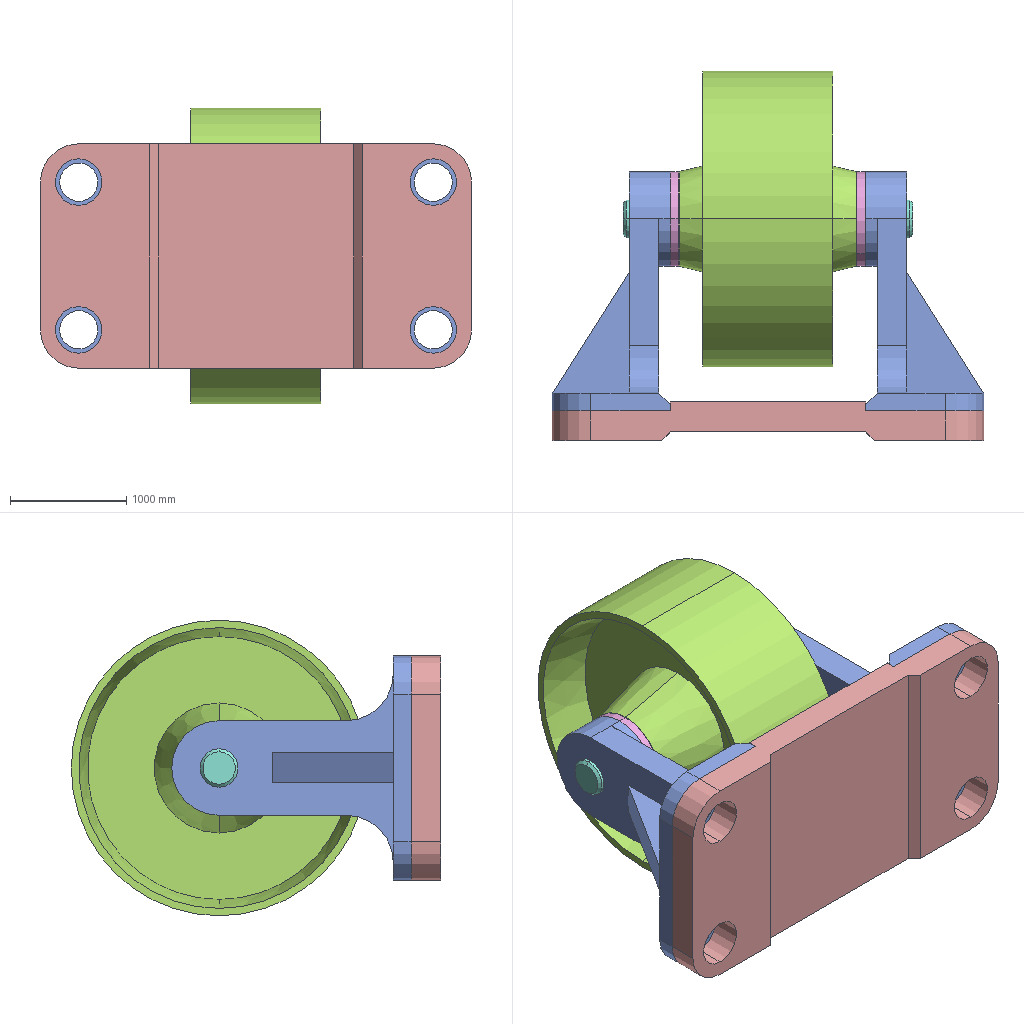Assembly | SolidWorks | 5 different items | 7 placed | box 3708 x 3175 x 2540 mm
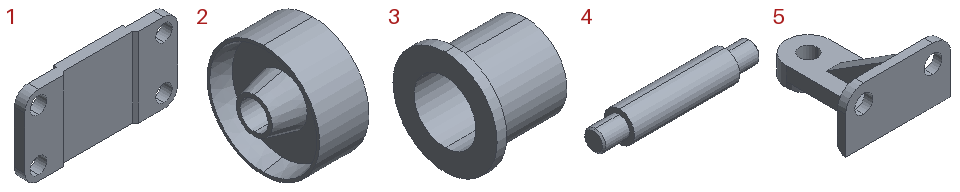Parts list (item | quantity | size | volume | features):
1 | x1 | 3708 x 330.2 x 1930 mm | 1654730858 mm3 | features ICE 3, Extrusion 1
2 | x1 | 1524 x 2540 x 2540 mm | 2412190480 mm3 | features Revolution 1
3 | x2 | 635 x 812.8 x 812.8 mm | 100350275 mm3 | features Revolution 1
4 | x1 | 2489 x 482.6 x 482.6 mm | 375617457 mm3 | features Chamfer 1, Revolution 1
5 | x2 | 1930 x 2057 x 1016 mm | 760890020 mm3 | features ICE 4, Chamfer 1, Extrusion 1, Fillet 1
Mates (type | each side: item.copy, entity, surface, feature):
Concentric | 1.1 face cylinder Boss-Extrude1 | 5.1 face cylinder Boss-Extrude1 | 2 times
Coincident | 1.1 face plane Boss-Extrude1 | 5.1 face plane Boss-Extrude1
Concentric | 1.1 face cylinder Boss-Extrude1 | 5.2 face cylinder Boss-Extrude1 | 2 times
Coincident | 1.1 face plane Boss-Extrude1 | 5.2 face plane Boss-Extrude1
Concentric | 5.1 edge | 3.1 face cylinder Revolve1
Coincident | 5.1 face plane Boss-Extrude4 | 3.1 face plane Revolve1
Concentric | 5.2 face cylinder Boss-Extrude3 | 3.2 face cylinder Revolve1
Coincident | 5.2 face plane Boss-Extrude4 | 3.2 face plane Revolve1
Concentric | 4.1 face cylinder Revolve1 | 3.1 face cylinder Revolve1
Width | 5.1 face plane Boss-Extrude3 | 5.2 face plane Boss-Extrude3 | 4.1 face plane Revolve1 | 4.1 face plane Revolve1
Concentric | 2.1 face cylinder Revolve1 | 3.2 face cylinder Revolve1